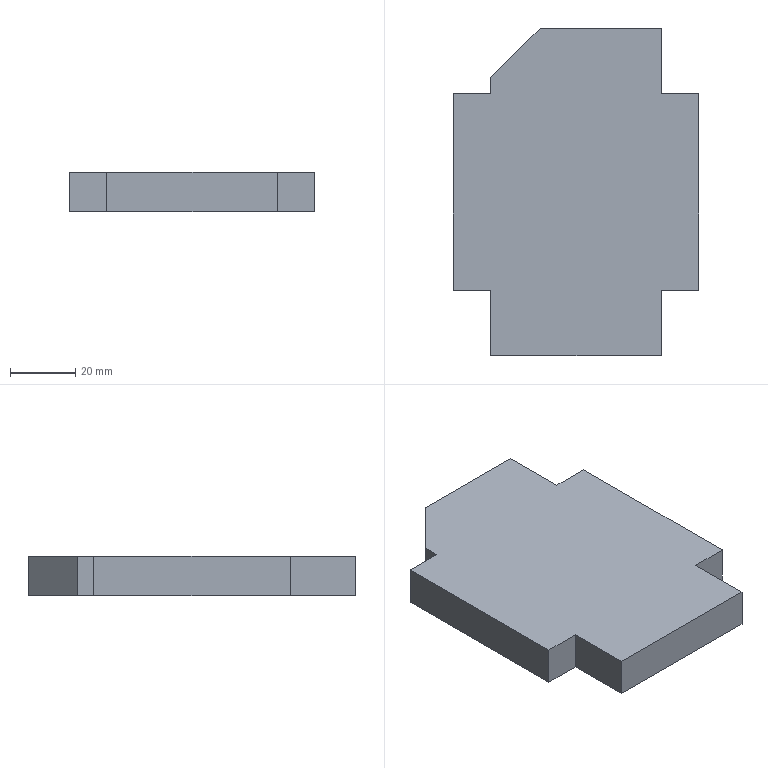Part | SolidWorks | features FlatPattern 1, SMBaseFlange 1, SheetMetal 1 | 1 solid | 15 faces | box 75 x 100 x 12 mm | volume 77610 mm3 | plane 15
STEP:
#1=CARTESIAN_POINT('',(296.937,-225.509,0.));
#2=VERTEX_POINT('',#1);
#3=CARTESIAN_POINT('',(296.937,-205.509,0.));
#4=VERTEX_POINT('',#3);
#5=CARTESIAN_POINT('',(296.937,-205.509,0.));
#6=DIRECTION('',(0.,1.,0.));
#7=VECTOR('',#6,1000.);
#8=LINE('',#5,#7);
#9=EDGE_CURVE('',#2,#4,#8,.T.);
#10=ORIENTED_EDGE('',*,*,#9,.F.);
#11=CARTESIAN_POINT('',(296.937,-225.509,-12.));
#12=VERTEX_POINT('',#11);
#13=CARTESIAN_POINT('',(296.937,-225.509,-12.));
#14=DIRECTION('',(0.,0.,1.));
#15=VECTOR('',#14,1000.);
#16=LINE('',#13,#15);
#17=EDGE_CURVE('',#12,#2,#16,.T.);
#18=ORIENTED_EDGE('',*,*,#17,.F.);
#19=CARTESIAN_POINT('',(296.937,-205.509,-12.));
#20=VERTEX_POINT('',#19);
#21=CARTESIAN_POINT('',(296.937,-205.509,-12.));
#22=DIRECTION('',(0.,1.,0.));
#23=VECTOR('',#22,1000.);
#24=LINE('',#21,#23);
#25=EDGE_CURVE('',#12,#20,#24,.T.);
#26=ORIENTED_EDGE('',*,*,#25,.T.);
#27=CARTESIAN_POINT('',(296.937,-205.509,-12.));
#28=DIRECTION('',(0.,0.,1.));
#29=VECTOR('',#28,1000.);
#30=LINE('',#27,#29);
#31=EDGE_CURVE('',#20,#4,#30,.T.);
#32=ORIENTED_EDGE('',*,*,#31,.T.);
#33=EDGE_LOOP('',(#10,#18,#26,#32));
#34=FACE_OUTER_BOUND('',#33,.T.);
#35=CARTESIAN_POINT('',(296.937,-205.509,-12.));
#36=DIRECTION('',(1.,0.,0.));
#37=DIRECTION('',(0.,0.,-1.));
#38=AXIS2_PLACEMENT_3D('',#35,#36,#37);
#39=PLANE('',#38);
#40=ADVANCED_FACE('',(#34),#39,.T.);
#41=CARTESIAN_POINT('',(308.437,-225.509,0.));
#42=VERTEX_POINT('',#41);
#43=CARTESIAN_POINT('',(296.937,-225.509,0.));
#44=DIRECTION('',(-1.,0.,0.));
#45=VECTOR('',#44,1000.);
#46=LINE('',#43,#45);
#47=EDGE_CURVE('',#42,#2,#46,.T.);
#48=ORIENTED_EDGE('',*,*,#47,.F.);
#49=CARTESIAN_POINT('',(308.437,-225.509,-12.));
#50=VERTEX_POINT('',#49);
#51=CARTESIAN_POINT('',(308.437,-225.509,-12.));
#52=DIRECTION('',(0.,0.,1.));
#53=VECTOR('',#52,1000.);
#54=LINE('',#51,#53);
#55=EDGE_CURVE('',#50,#42,#54,.T.);
#56=ORIENTED_EDGE('',*,*,#55,.F.);
#57=CARTESIAN_POINT('',(296.937,-225.509,-12.));
#58=DIRECTION('',(-1.,0.,0.));
#59=VECTOR('',#58,1000.);
#60=LINE('',#57,#59);
#61=EDGE_CURVE('',#50,#12,#60,.T.);
#62=ORIENTED_EDGE('',*,*,#61,.T.);
#63=ORIENTED_EDGE('',*,*,#17,.T.);
#64=EDGE_LOOP('',(#48,#56,#62,#63));
#65=FACE_OUTER_BOUND('',#64,.T.);
#66=CARTESIAN_POINT('',(296.937,-225.509,-12.));
#67=DIRECTION('',(0.,1.,0.));
#68=DIRECTION('',(0.,0.,1.));
#69=AXIS2_PLACEMENT_3D('',#66,#67,#68);
#70=PLANE('',#69);
#71=ADVANCED_FACE('',(#65),#70,.T.);
#72=CARTESIAN_POINT('',(308.437,-285.509,0.));
#73=VERTEX_POINT('',#72);
#74=CARTESIAN_POINT('',(308.437,-225.509,0.));
#75=DIRECTION('',(0.,1.,0.));
#76=VECTOR('',#75,1000.);
#77=LINE('',#74,#76);
#78=EDGE_CURVE('',#73,#42,#77,.T.);
#79=ORIENTED_EDGE('',*,*,#78,.F.);
#80=CARTESIAN_POINT('',(308.437,-285.509,-12.));
#81=VERTEX_POINT('',#80);
#82=CARTESIAN_POINT('',(308.437,-285.509,-12.));
#83=DIRECTION('',(0.,0.,1.));
#84=VECTOR('',#83,1000.);
#85=LINE('',#82,#84);
#86=EDGE_CURVE('',#81,#73,#85,.T.);
#87=ORIENTED_EDGE('',*,*,#86,.F.);
#88=CARTESIAN_POINT('',(308.437,-225.509,-12.));
#89=DIRECTION('',(0.,1.,0.));
#90=VECTOR('',#89,1000.);
#91=LINE('',#88,#90);
#92=EDGE_CURVE('',#81,#50,#91,.T.);
#93=ORIENTED_EDGE('',*,*,#92,.T.);
#94=ORIENTED_EDGE('',*,*,#55,.T.);
#95=EDGE_LOOP('',(#79,#87,#93,#94));
#96=FACE_OUTER_BOUND('',#95,.T.);
#97=CARTESIAN_POINT('',(308.437,-225.509,-12.));
#98=DIRECTION('',(1.,0.,0.));
#99=DIRECTION('',(0.,0.,-1.));
#100=AXIS2_PLACEMENT_3D('',#97,#98,#99);
#101=PLANE('',#100);
#102=ADVANCED_FACE('',(#96),#101,.T.);
#103=CARTESIAN_POINT('',(296.937,-285.509,0.));
#104=VERTEX_POINT('',#103);
#105=CARTESIAN_POINT('',(308.437,-285.509,0.));
#106=DIRECTION('',(1.,0.,0.));
#107=VECTOR('',#106,1000.);
#108=LINE('',#105,#107);
#109=EDGE_CURVE('',#104,#73,#108,.T.);
#110=ORIENTED_EDGE('',*,*,#109,.F.);
#111=CARTESIAN_POINT('',(296.937,-285.509,-12.));
#112=VERTEX_POINT('',#111);
#113=CARTESIAN_POINT('',(296.937,-285.509,-12.));
#114=DIRECTION('',(0.,0.,1.));
#115=VECTOR('',#114,1000.);
#116=LINE('',#113,#115);
#117=EDGE_CURVE('',#112,#104,#116,.T.);
#118=ORIENTED_EDGE('',*,*,#117,.F.);
#119=CARTESIAN_POINT('',(308.437,-285.509,-12.));
#120=DIRECTION('',(1.,0.,0.));
#121=VECTOR('',#120,1000.);
#122=LINE('',#119,#121);
#123=EDGE_CURVE('',#112,#81,#122,.T.);
#124=ORIENTED_EDGE('',*,*,#123,.T.);
#125=ORIENTED_EDGE('',*,*,#86,.T.);
#126=EDGE_LOOP('',(#110,#118,#124,#125));
#127=FACE_OUTER_BOUND('',#126,.T.);
#128=CARTESIAN_POINT('',(308.437,-285.509,-12.));
#129=DIRECTION('',(0.,-1.,0.));
#130=DIRECTION('',(1.,0.,0.));
#131=AXIS2_PLACEMENT_3D('',#128,#129,#130);
#132=PLANE('',#131);
#133=ADVANCED_FACE('',(#127),#132,.T.);
#134=CARTESIAN_POINT('',(296.937,-305.509,0.));
#135=VERTEX_POINT('',#134);
#136=CARTESIAN_POINT('',(296.937,-285.509,0.));
#137=DIRECTION('',(0.,1.,0.));
#138=VECTOR('',#137,1000.);
#139=LINE('',#136,#138);
#140=EDGE_CURVE('',#135,#104,#139,.T.);
#141=ORIENTED_EDGE('',*,*,#140,.F.);
#142=CARTESIAN_POINT('',(296.937,-305.509,-12.));
#143=VERTEX_POINT('',#142);
#144=CARTESIAN_POINT('',(296.937,-305.509,-12.));
#145=DIRECTION('',(0.,0.,1.));
#146=VECTOR('',#145,1000.);
#147=LINE('',#144,#146);
#148=EDGE_CURVE('',#143,#135,#147,.T.);
#149=ORIENTED_EDGE('',*,*,#148,.F.);
#150=CARTESIAN_POINT('',(296.937,-285.509,-12.));
#151=DIRECTION('',(0.,1.,0.));
#152=VECTOR('',#151,1000.);
#153=LINE('',#150,#152);
#154=EDGE_CURVE('',#143,#112,#153,.T.);
#155=ORIENTED_EDGE('',*,*,#154,.T.);
#156=ORIENTED_EDGE('',*,*,#117,.T.);
#157=EDGE_LOOP('',(#141,#149,#155,#156));
#158=FACE_OUTER_BOUND('',#157,.T.);
#159=CARTESIAN_POINT('',(296.937,-285.509,-12.));
#160=DIRECTION('',(1.,0.,0.));
#161=DIRECTION('',(0.,0.,-1.));
#162=AXIS2_PLACEMENT_3D('',#159,#160,#161);
#163=PLANE('',#162);
#164=ADVANCED_FACE('',(#158),#163,.T.);
#165=CARTESIAN_POINT('',(244.937,-305.509,0.));
#166=VERTEX_POINT('',#165);
#167=CARTESIAN_POINT('',(296.937,-305.509,0.));
#168=DIRECTION('',(1.,0.,0.));
#169=VECTOR('',#168,1000.);
#170=LINE('',#167,#169);
#171=EDGE_CURVE('',#166,#135,#170,.T.);
#172=ORIENTED_EDGE('',*,*,#171,.F.);
#173=CARTESIAN_POINT('',(244.937,-305.509,-12.));
#174=VERTEX_POINT('',#173);
#175=CARTESIAN_POINT('',(244.937,-305.509,-12.));
#176=DIRECTION('',(0.,0.,1.));
#177=VECTOR('',#176,1000.);
#178=LINE('',#175,#177);
#179=EDGE_CURVE('',#174,#166,#178,.T.);
#180=ORIENTED_EDGE('',*,*,#179,.F.);
#181=CARTESIAN_POINT('',(296.937,-305.509,-12.));
#182=DIRECTION('',(1.,0.,0.));
#183=VECTOR('',#182,1000.);
#184=LINE('',#181,#183);
#185=EDGE_CURVE('',#174,#143,#184,.T.);
#186=ORIENTED_EDGE('',*,*,#185,.T.);
#187=ORIENTED_EDGE('',*,*,#148,.T.);
#188=EDGE_LOOP('',(#172,#180,#186,#187));
#189=FACE_OUTER_BOUND('',#188,.T.);
#190=CARTESIAN_POINT('',(296.937,-305.509,-12.));
#191=DIRECTION('',(0.,-1.,0.));
#192=DIRECTION('',(0.,0.,-1.));
#193=AXIS2_PLACEMENT_3D('',#190,#191,#192);
#194=PLANE('',#193);
#195=ADVANCED_FACE('',(#189),#194,.T.);
#196=CARTESIAN_POINT('',(244.937,-285.509,0.));
#197=VERTEX_POINT('',#196);
#198=CARTESIAN_POINT('',(244.937,-285.509,0.));
#199=DIRECTION('',(0.,-1.,0.));
#200=VECTOR('',#199,1000.);
#201=LINE('',#198,#200);
#202=EDGE_CURVE('',#197,#166,#201,.T.);
#203=ORIENTED_EDGE('',*,*,#202,.F.);
#204=CARTESIAN_POINT('',(244.937,-285.509,-12.));
#205=VERTEX_POINT('',#204);
#206=CARTESIAN_POINT('',(244.937,-285.509,-12.));
#207=DIRECTION('',(0.,0.,1.));
#208=VECTOR('',#207,1000.);
#209=LINE('',#206,#208);
#210=EDGE_CURVE('',#205,#197,#209,.T.);
#211=ORIENTED_EDGE('',*,*,#210,.F.);
#212=CARTESIAN_POINT('',(244.937,-285.509,-12.));
#213=DIRECTION('',(0.,-1.,0.));
#214=VECTOR('',#213,1000.);
#215=LINE('',#212,#214);
#216=EDGE_CURVE('',#205,#174,#215,.T.);
#217=ORIENTED_EDGE('',*,*,#216,.T.);
#218=ORIENTED_EDGE('',*,*,#179,.T.);
#219=EDGE_LOOP('',(#203,#211,#217,#218));
#220=FACE_OUTER_BOUND('',#219,.T.);
#221=CARTESIAN_POINT('',(244.937,-285.509,-12.));
#222=DIRECTION('',(-1.,0.,0.));
#223=DIRECTION('',(0.,0.,1.));
#224=AXIS2_PLACEMENT_3D('',#221,#222,#223);
#225=PLANE('',#224);
#226=ADVANCED_FACE('',(#220),#225,.T.);
#227=CARTESIAN_POINT('',(233.437,-285.509,0.));
#228=VERTEX_POINT('',#227);
#229=CARTESIAN_POINT('',(233.437,-285.509,0.));
#230=DIRECTION('',(1.,0.,0.));
#231=VECTOR('',#230,1000.);
#232=LINE('',#229,#231);
#233=EDGE_CURVE('',#228,#197,#232,.T.);
#234=ORIENTED_EDGE('',*,*,#233,.F.);
#235=CARTESIAN_POINT('',(233.437,-285.509,-12.));
#236=VERTEX_POINT('',#235);
#237=CARTESIAN_POINT('',(233.437,-285.509,-12.));
#238=DIRECTION('',(0.,0.,1.));
#239=VECTOR('',#238,1000.);
#240=LINE('',#237,#239);
#241=EDGE_CURVE('',#236,#228,#240,.T.);
#242=ORIENTED_EDGE('',*,*,#241,.F.);
#243=CARTESIAN_POINT('',(233.437,-285.509,-12.));
#244=DIRECTION('',(1.,0.,0.));
#245=VECTOR('',#244,1000.);
#246=LINE('',#243,#245);
#247=EDGE_CURVE('',#236,#205,#246,.T.);
#248=ORIENTED_EDGE('',*,*,#247,.T.);
#249=ORIENTED_EDGE('',*,*,#210,.T.);
#250=EDGE_LOOP('',(#234,#242,#248,#249));
#251=FACE_OUTER_BOUND('',#250,.T.);
#252=CARTESIAN_POINT('',(233.437,-285.509,-12.));
#253=DIRECTION('',(0.,-1.,0.));
#254=DIRECTION('',(0.,0.,-1.));
#255=AXIS2_PLACEMENT_3D('',#252,#253,#254);
#256=PLANE('',#255);
#257=ADVANCED_FACE('',(#251),#256,.T.);
#258=CARTESIAN_POINT('',(233.437,-225.509,0.));
#259=VERTEX_POINT('',#258);
#260=CARTESIAN_POINT('',(233.437,-225.509,0.));
#261=DIRECTION('',(0.,-1.,0.));
#262=VECTOR('',#261,1000.);
#263=LINE('',#260,#262);
#264=EDGE_CURVE('',#259,#228,#263,.T.);
#265=ORIENTED_EDGE('',*,*,#264,.F.);
#266=CARTESIAN_POINT('',(233.437,-225.509,-12.));
#267=VERTEX_POINT('',#266);
#268=CARTESIAN_POINT('',(233.437,-225.509,-12.));
#269=DIRECTION('',(0.,0.,1.));
#270=VECTOR('',#269,1000.);
#271=LINE('',#268,#270);
#272=EDGE_CURVE('',#267,#259,#271,.T.);
#273=ORIENTED_EDGE('',*,*,#272,.F.);
#274=CARTESIAN_POINT('',(233.437,-225.509,-12.));
#275=DIRECTION('',(0.,-1.,0.));
#276=VECTOR('',#275,1000.);
#277=LINE('',#274,#276);
#278=EDGE_CURVE('',#267,#236,#277,.T.);
#279=ORIENTED_EDGE('',*,*,#278,.T.);
#280=ORIENTED_EDGE('',*,*,#241,.T.);
#281=EDGE_LOOP('',(#265,#273,#279,#280));
#282=FACE_OUTER_BOUND('',#281,.T.);
#283=CARTESIAN_POINT('',(233.437,-225.509,-12.));
#284=DIRECTION('',(-1.,0.,0.));
#285=DIRECTION('',(0.,0.,1.));
#286=AXIS2_PLACEMENT_3D('',#283,#284,#285);
#287=PLANE('',#286);
#288=ADVANCED_FACE('',(#282),#287,.T.);
#289=CARTESIAN_POINT('',(244.937,-225.509,0.));
#290=VERTEX_POINT('',#289);
#291=CARTESIAN_POINT('',(244.937,-225.509,0.));
#292=DIRECTION('',(-1.,0.,0.));
#293=VECTOR('',#292,1000.);
#294=LINE('',#291,#293);
#295=EDGE_CURVE('',#290,#259,#294,.T.);
#296=ORIENTED_EDGE('',*,*,#295,.F.);
#297=CARTESIAN_POINT('',(244.937,-225.509,-12.));
#298=VERTEX_POINT('',#297);
#299=CARTESIAN_POINT('',(244.937,-225.509,-12.));
#300=DIRECTION('',(0.,0.,1.));
#301=VECTOR('',#300,1000.);
#302=LINE('',#299,#301);
#303=EDGE_CURVE('',#298,#290,#302,.T.);
#304=ORIENTED_EDGE('',*,*,#303,.F.);
#305=CARTESIAN_POINT('',(244.937,-225.509,-12.));
#306=DIRECTION('',(-1.,0.,0.));
#307=VECTOR('',#306,1000.);
#308=LINE('',#305,#307);
#309=EDGE_CURVE('',#298,#267,#308,.T.);
#310=ORIENTED_EDGE('',*,*,#309,.T.);
#311=ORIENTED_EDGE('',*,*,#272,.T.);
#312=EDGE_LOOP('',(#296,#304,#310,#311));
#313=FACE_OUTER_BOUND('',#312,.T.);
#314=CARTESIAN_POINT('',(244.937,-225.509,-12.));
#315=DIRECTION('',(0.,1.,0.));
#316=DIRECTION('',(0.,0.,1.));
#317=AXIS2_PLACEMENT_3D('',#314,#315,#316);
#318=PLANE('',#317);
#319=ADVANCED_FACE('',(#313),#318,.T.);
#320=CARTESIAN_POINT('',(244.937,-220.509,0.));
#321=VERTEX_POINT('',#320);
#322=CARTESIAN_POINT('',(244.937,-220.509,0.));
#323=DIRECTION('',(0.,-1.,0.));
#324=VECTOR('',#323,1000.);
#325=LINE('',#322,#324);
#326=EDGE_CURVE('',#321,#290,#325,.T.);
#327=ORIENTED_EDGE('',*,*,#326,.F.);
#328=CARTESIAN_POINT('',(244.937,-220.509,-12.));
#329=VERTEX_POINT('',#328);
#330=CARTESIAN_POINT('',(244.937,-220.509,-12.));
#331=DIRECTION('',(0.,0.,1.));
#332=VECTOR('',#331,1000.);
#333=LINE('',#330,#332);
#334=EDGE_CURVE('',#329,#321,#333,.T.);
#335=ORIENTED_EDGE('',*,*,#334,.F.);
#336=CARTESIAN_POINT('',(244.937,-220.509,-12.));
#337=DIRECTION('',(0.,-1.,0.));
#338=VECTOR('',#337,1000.);
#339=LINE('',#336,#338);
#340=EDGE_CURVE('',#329,#298,#339,.T.);
#341=ORIENTED_EDGE('',*,*,#340,.T.);
#342=ORIENTED_EDGE('',*,*,#303,.T.);
#343=EDGE_LOOP('',(#327,#335,#341,#342));
#344=FACE_OUTER_BOUND('',#343,.T.);
#345=CARTESIAN_POINT('',(244.937,-220.509,-12.));
#346=DIRECTION('',(-1.,0.,0.));
#347=DIRECTION('',(0.,-1.,0.));
#348=AXIS2_PLACEMENT_3D('',#345,#346,#347);
#349=PLANE('',#348);
#350=ADVANCED_FACE('',(#344),#349,.T.);
#351=CARTESIAN_POINT('',(259.937,-205.509,0.));
#352=VERTEX_POINT('',#351);
#353=CARTESIAN_POINT('',(259.937,-205.509,0.));
#354=DIRECTION('',(-0.7071,-0.7071,0.));
#355=VECTOR('',#354,1000.);
#356=LINE('',#353,#355);
#357=EDGE_CURVE('',#352,#321,#356,.T.);
#358=ORIENTED_EDGE('',*,*,#357,.F.);
#359=CARTESIAN_POINT('',(259.937,-205.509,-12.));
#360=VERTEX_POINT('',#359);
#361=CARTESIAN_POINT('',(259.937,-205.509,-12.));
#362=DIRECTION('',(0.,0.,1.));
#363=VECTOR('',#362,1000.);
#364=LINE('',#361,#363);
#365=EDGE_CURVE('',#360,#352,#364,.T.);
#366=ORIENTED_EDGE('',*,*,#365,.F.);
#367=CARTESIAN_POINT('',(259.937,-205.509,-12.));
#368=DIRECTION('',(-0.7071,-0.7071,0.));
#369=VECTOR('',#368,1000.);
#370=LINE('',#367,#369);
#371=EDGE_CURVE('',#360,#329,#370,.T.);
#372=ORIENTED_EDGE('',*,*,#371,.T.);
#373=ORIENTED_EDGE('',*,*,#334,.T.);
#374=EDGE_LOOP('',(#358,#366,#372,#373));
#375=FACE_OUTER_BOUND('',#374,.T.);
#376=CARTESIAN_POINT('',(259.937,-205.509,-12.));
#377=DIRECTION('',(-0.7071,0.7071,0.));
#378=DIRECTION('',(-0.7071,-0.7071,0.));
#379=AXIS2_PLACEMENT_3D('',#376,#377,#378);
#380=PLANE('',#379);
#381=ADVANCED_FACE('',(#375),#380,.T.);
#382=CARTESIAN_POINT('',(296.937,-205.509,0.));
#383=DIRECTION('',(-1.,0.,0.));
#384=VECTOR('',#383,1000.);
#385=LINE('',#382,#384);
#386=EDGE_CURVE('',#4,#352,#385,.T.);
#387=ORIENTED_EDGE('',*,*,#386,.F.);
#388=ORIENTED_EDGE('',*,*,#31,.F.);
#389=CARTESIAN_POINT('',(296.937,-205.509,-12.));
#390=DIRECTION('',(-1.,0.,0.));
#391=VECTOR('',#390,1000.);
#392=LINE('',#389,#391);
#393=EDGE_CURVE('',#20,#360,#392,.T.);
#394=ORIENTED_EDGE('',*,*,#393,.T.);
#395=ORIENTED_EDGE('',*,*,#365,.T.);
#396=EDGE_LOOP('',(#387,#388,#394,#395));
#397=FACE_OUTER_BOUND('',#396,.T.);
#398=CARTESIAN_POINT('',(296.937,-205.509,-12.));
#399=DIRECTION('',(0.,1.,0.));
#400=DIRECTION('',(0.,0.,1.));
#401=AXIS2_PLACEMENT_3D('',#398,#399,#400);
#402=PLANE('',#401);
#403=ADVANCED_FACE('',(#397),#402,.T.);
#404=ORIENTED_EDGE('',*,*,#25,.F.);
#405=ORIENTED_EDGE('',*,*,#61,.F.);
#406=ORIENTED_EDGE('',*,*,#92,.F.);
#407=ORIENTED_EDGE('',*,*,#123,.F.);
#408=ORIENTED_EDGE('',*,*,#154,.F.);
#409=ORIENTED_EDGE('',*,*,#185,.F.);
#410=ORIENTED_EDGE('',*,*,#216,.F.);
#411=ORIENTED_EDGE('',*,*,#247,.F.);
#412=ORIENTED_EDGE('',*,*,#278,.F.);
#413=ORIENTED_EDGE('',*,*,#309,.F.);
#414=ORIENTED_EDGE('',*,*,#340,.F.);
#415=ORIENTED_EDGE('',*,*,#371,.F.);
#416=ORIENTED_EDGE('',*,*,#393,.F.);
#417=EDGE_LOOP('',(#404,#405,#406,#407,#408,#409,#410,#411,#412,#413,#414,#415,#416));
#418=FACE_OUTER_BOUND('',#417,.T.);
#419=CARTESIAN_POINT('',(0.,0.,-12.));
#420=DIRECTION('',(0.,0.,1.));
#421=DIRECTION('',(1.,0.,0.));
#422=AXIS2_PLACEMENT_3D('',#419,#420,#421);
#423=PLANE('',#422);
#424=ADVANCED_FACE('',(#418),#423,.F.);
#425=ORIENTED_EDGE('',*,*,#9,.T.);
#426=ORIENTED_EDGE('',*,*,#386,.T.);
#427=ORIENTED_EDGE('',*,*,#357,.T.);
#428=ORIENTED_EDGE('',*,*,#326,.T.);
#429=ORIENTED_EDGE('',*,*,#295,.T.);
#430=ORIENTED_EDGE('',*,*,#264,.T.);
#431=ORIENTED_EDGE('',*,*,#233,.T.);
#432=ORIENTED_EDGE('',*,*,#202,.T.);
#433=ORIENTED_EDGE('',*,*,#171,.T.);
#434=ORIENTED_EDGE('',*,*,#140,.T.);
#435=ORIENTED_EDGE('',*,*,#109,.T.);
#436=ORIENTED_EDGE('',*,*,#78,.T.);
#437=ORIENTED_EDGE('',*,*,#47,.T.);
#438=EDGE_LOOP('',(#425,#426,#427,#428,#429,#430,#431,#432,#433,#434,#435,#436,#437));
#439=FACE_OUTER_BOUND('',#438,.T.);
#440=CARTESIAN_POINT('',(0.,0.,0.));
#441=DIRECTION('',(0.,0.,1.));
#442=DIRECTION('',(1.,0.,0.));
#443=AXIS2_PLACEMENT_3D('',#440,#441,#442);
#444=PLANE('',#443);
#445=ADVANCED_FACE('',(#439),#444,.T.);
#446=CLOSED_SHELL('',(#40,#71,#102,#133,#164,#195,#226,#257,#288,#319,#350,#381,#403,#424,#445));
#447=MANIFOLD_SOLID_BREP('',#446);
#448=CARTESIAN_POINT('',(0.,0.,0.));
#449=DIRECTION('',(0.,0.,1.));
#450=DIRECTION('',(1.,0.,0.));
#451=AXIS2_PLACEMENT_3D('',#448,#449,#450);
#452=(LENGTH_UNIT()NAMED_UNIT(*)SI_UNIT(.MILLI.,.METRE.));
#453=UNCERTAINTY_MEASURE_WITH_UNIT(LENGTH_MEASURE(0.00001),#452,'','');
#454=(NAMED_UNIT(*)PLANE_ANGLE_UNIT()SI_UNIT($,.RADIAN.));
#455=(NAMED_UNIT(*)SI_UNIT($,.STERADIAN.)SOLID_ANGLE_UNIT());
#456=(GEOMETRIC_REPRESENTATION_CONTEXT(3)GLOBAL_UNCERTAINTY_ASSIGNED_CONTEXT((#453))GLOBAL_UNIT_ASSIGNED_CONTEXT((#452,#454,#455))REPRESENTATION_CONTEXT('',''));
#457=ADVANCED_BREP_SHAPE_REPRESENTATION('',(#447,#451),#456);